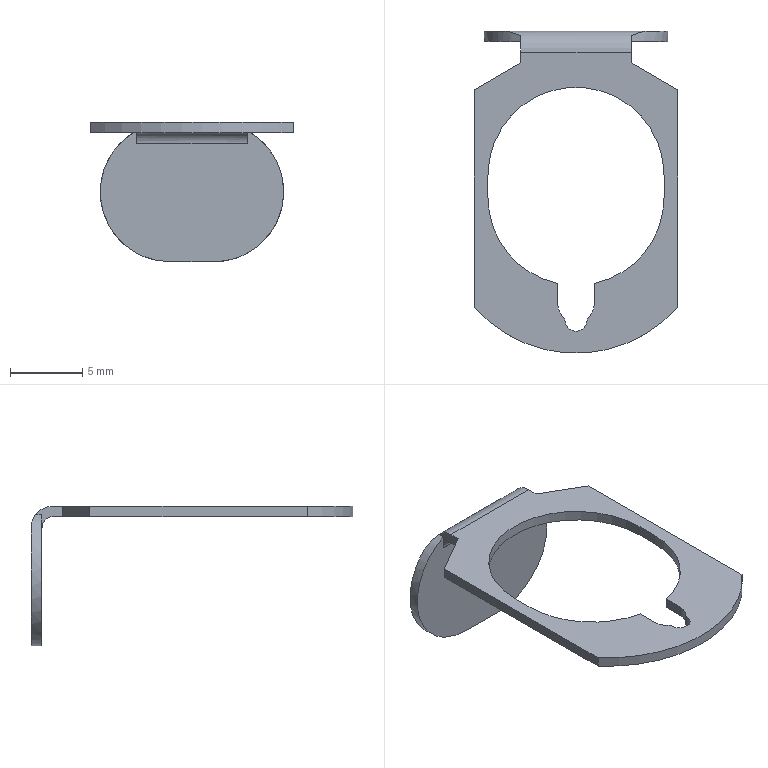Part | SolidWorks | features BaseBody 1 | 1 solid | 84 faces | box 14.097 x 22.301 x 9.652 mm | volume 165.496 mm3 | plane 67 | cylinder 17 | commonest cylinder face diameters 12.192 x3 1.524 x2 2.54 x2 9.652 x2 0.209 x1 0.514 x1